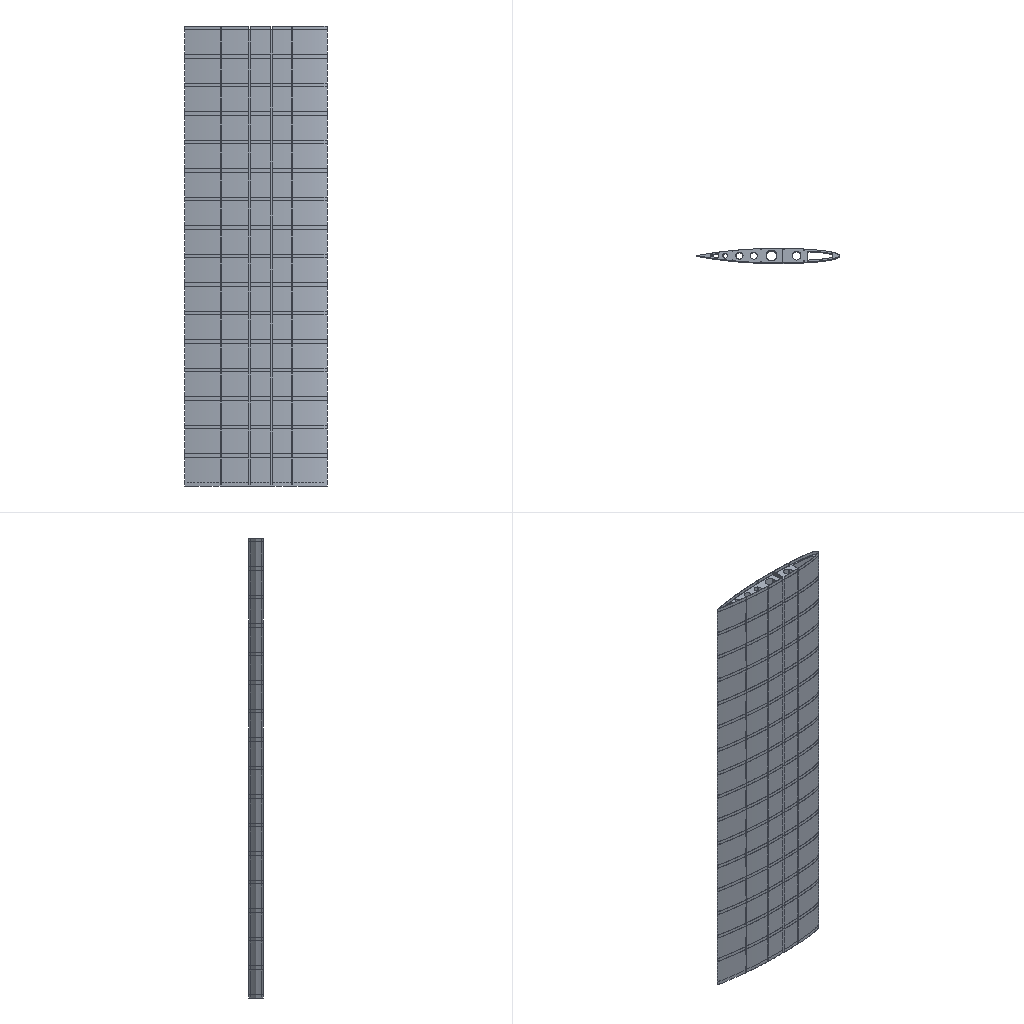Simulation study | abaqus
Set-up summary:
category,name,step,type,value,unit,region
solver,abaqus
solver,version,,,Abaqus/Standard 2020
units,not stated in the deck,,not stated
analysis,deck,,static,static
load_step,Step-1,Step-1,static,nlgeom=True
contact,interactions,,,general=0 pairs=0 ties=0
load_step,requested,,,1
mesh,nodes,,,93184
mesh,elements,,,87242
element_type,S3,,shell,1575
element_type,S4R,,shell,85667
load,load commands in deck,,count,1
bc,support commands in deck,,count,1
material,MATERIAL-1,,in results
check,setup vs results,,match,"per instance, exact: element labels, types and connectivity; labels of the nodes the elements use; coordinates of those nodes at SINGLE_PRECISION in 1 of 1 instance(s)"
Abaqus input file, long lists of numbers shortened:
*Heading
** Job name: Job-2 Model name: Job-15872
** Generated by: Abaqus/CAE 2020
*Preprint, echo=NO, model=NO, history=NO, contact=NO
**
** PARTS
**
*Part, name=PART-4
*Node
      1,  -108.057,  -2.084,           5.
      2,  -110.05,  -1.754,           5.
** (93182 more lines like these left out)
*Element, type=S4R
  1, 58648, 58655, 57835, 57834
  2, 58655, 58656, 57836, 57835
** (85665 more lines like these left out)
*Element, type=S3
271, 90430, 90428, 91111
272, 75408, 75407, 73694
** (1573 more lines like these left out)
*Nset, nset=SET-1
     4,     5,     6,    13,    14,    15,    16,    17,    18,    19,    20,    21,    22,    23,    24,    25
    26,    52,    53,    54,    55,    56,    57,    58,    59,    60,    61,    62,    63,    64,    90,    91
** (2480 more lines like these left out)
*Elset, elset=SET-1
   906,   907,   908,   909,   910,   911,   912,   913,   914,   915,   916,   917,   918,   919,   920,   921
   922,   923,   924,   925,   926,   927,   928,   929,   930,   931,   932,   933,   934,   935,   936,   937
** (2295 more lines like these left out)
*Nset, nset=SET-2
 50078, 50081, 50082, 50090, 50107, 50108, 50110, 50111, 50112, 50121, 50122, 50123, 50223, 50224, 50226, 50227
 50228, 50237, 50238, 50239, 50337, 50338, 50340, 50341, 50342, 50351, 50352, 50353, 50451, 50452, 50454, 50457
** (1104 more lines like these left out)
*Elset, elset=SET-2
   271,   272,   273,   274,   275,   276,   277,   278,   279,   280,   281,   282,   283,   284,   285,   286
   287,   288,   289,   290,   291,   292,   293,   294,   295,   296,   297,   298,   299,   300,   301,   302
** (951 more lines like these left out)
*Nset, nset=SET-8
   622,   636,   660,   705,   737,   773,   805,   841,   880,   909,   948,   977,  1016,  1045,  1091,  1113
  1159,  1181,  1227,  1249,  1302,  1317,  1370,  1385,  1438,  1453,  1513,  1521,  1581,  1589,  1649,  1657
** (317 more lines like these left out)
*Elset, elset=SET-8
   729,   730,   731,   732,   733,   734,   735,   736,   737,   738,   739,   740,   741,   742,   743,   744
   745,   746,   747,   748,   749,   750,   751,   752,   753,   754,   755,   756,   757,   758,   759,   760
** (258 more lines like these left out)
*Nset, nset=SET-9
     1,     2,     3,     4,     5,     6,     7,     8,     9,    10,    11,    12,    13,    14,    15,    16
    17,    27,    28,    29,    30,    31,    32,    33,    34,    35,    36,    37,    38,    39,    40,    41
** (317 more lines like these left out)
*Elset, elset=SET-9
   654,   655,   656,   657,   658,   659,   660,   661,   662,   663,   664,   665,   666,   667,   668,   669
   670,   671,   672,   673,   674,   675,   676,   677,   678,   679,   680,   681,   682,   683,   684,   685
** (258 more lines like these left out)
*Nset, nset=SET-10
 22694, 22695, 22700, 22701, 22702, 22703, 22704, 22705, 22711, 22714, 22715, 22716, 22742, 22747, 22748, 22749
 22750, 22751, 22752, 22753, 22754, 22755, 22756, 22757, 22758, 22759, 22760, 22761, 22762, 22763, 22764, 22765
** (244 more lines like these left out)
*Elset, elset=SET-10
   804,   805,   806,   807,   808,   809,   810,   811,   812,   813,   814,   815,   816,   817,   818,   819
   820,   821,   822,   823,   824,   825,   826,   827,   828,   829,   830,   831,   832,   833,   834,   835
** (197 more lines like these left out)
*Nset, nset=SET-11
 18342, 18343, 18344, 18345, 18346, 18347, 18348, 18349, 18350, 18351, 18352, 18353, 18354, 18355, 18356, 18357
 18358, 18359, 18360, 18361, 18371, 18372, 18373, 18374, 18375, 18376, 18377, 18378, 18379, 18380, 18381, 18382
** (243 more lines like these left out)
*Elset, elset=SET-11
   603,   604,   605,   606,   607,   608,   609,   610,   611,   612,   613,   614,   615,   616,   617,   618
   619,   620,   621,   622,   623,   624,   625,   626,   627,   628,   629,   630,   631,   632,   633,   634
** (197 more lines like these left out)
*Nset, nset=SET-12
 43563, 43564, 43571, 43572, 43573, 43574, 43575, 43576, 43577, 43578, 43579, 43580, 43583, 43584, 43585, 43586
 43587, 43588, 43589, 43590, 43593, 43598, 43599, 43600, 43601, 43602, 43603, 43604, 43605, 43645, 43652, 43653
** (176 more lines like these left out)
*Elset, elset=SET-12
   864,   865,   866,   867,   868,   869,   870,   871,   872,   873,   874,   875,   876,   877,   878,   879
   880,   881,   882,   883,   884,   885,   886,   887,   888,   889,   890,   891,   892,   893,   894,   895
** (141 more lines like these left out)
*Nset, nset=SET-13
 37577, 37578, 37583, 37584, 37585, 37586, 37587, 37588, 37589, 37590, 37591, 37592, 37597, 37598, 37599, 37600
 37601, 37602, 37603, 37604, 37608, 37612, 37613, 37614, 37615, 37616, 37617, 37618, 37619, 37661, 37663, 37664
** (176 more lines like these left out)
*Elset, elset=SET-13
   561,   562,   563,   564,   565,   566,   567,   568,   569,   570,   571,   572,   573,   574,   575,   576
   577,   578,   579,   580,   581,   582,   583,   584,   585,   586,   587,   588,   589,   590,   591,   592
** (141 more lines like these left out)
*Nset, nset=SET-14
 58650, 58651, 58657, 58658, 58659, 58660, 58669, 58670, 58678, 58681, 58682, 58729, 58735, 58736, 58737, 58738
 58739, 58740, 58753, 58754, 58755, 58756, 58757, 58758, 58759, 58760, 58794, 58797, 58798, 58843, 58849, 58850
** (176 more lines like these left out)
*Elset, elset=SET-14
    31,    32,    33,    34,    35,    36,    37,    38,    39,    40,    41,    42,    43,    44,    45,    46
    47,    48,    49,    50,    51,    52,    53,    54,    55,    56,    57,    58,    59,    60,    61,    62
** (141 more lines like these left out)
*Nset, nset=SET-15
 50080, 50081, 50087, 50088, 50089, 50090, 50099, 50100, 50108, 50111, 50112, 50159, 50165, 50166, 50167, 50168
 50169, 50170, 50183, 50184, 50185, 50186, 50187, 50188, 50189, 50190, 50224, 50227, 50228, 50273, 50279, 50280
** (176 more lines like these left out)
*Elset, elset=SET-15
   229,   230,   231,   232,   233,   234,   235,   236,   237,   238,   239,   240,   241,   242,   243,   244
   245,   246,   247,   248,   249,   250,   251,   252,   253,   254,   255,   256,   257,   258,   259,   260
** (141 more lines like these left out)
*Nset, nset=SET-16
 73686, 73687, 73690, 73691, 73692, 73693, 73694, 73695, 73696, 73697, 73700, 73701, 73702, 73703, 73704, 73705
 73706, 73708, 73709, 73710, 73711, 73712, 73713, 73725, 73727, 73728, 73729, 73730, 73731, 73732, 73733, 73734
** (618 more lines like these left out)
*Elset, elset=SET-16
    73,    74,    75,    76,    77,    78,    79,    80,    81,    82,    83,    84,    85,    86,    87,    88
    89,    90,    91,    92,    93,    94,    95,    96,    97,    98,    99,   100,   101,   102,   103,   104
** (508 more lines like these left out)
*Nset, nset=SET-17
 50078, 50079, 50085, 50086, 50107, 50158, 50161, 50162, 50163, 50164, 50223, 50272, 50275, 50276, 50277, 50278
 50337, 50386, 50389, 50390, 50391, 50392, 50451, 50455, 50513, 50516, 50517, 50518, 50565, 50569, 50627, 50630
** (115 more lines like these left out)
*Elset, elset=SET-17
     1,     2,     3,     4,     5,     6,     7,     8,     9,    10,    11,    12,    13,    14,    15,    16
    17,    18,    19,    20,    21,    22,    23,    24,    25,    26,    27,    28,    29,    30,  1387,  1388
** (90 more lines like these left out)
*Nset, nset=SET-18
 50083, 50084, 50091, 50092, 50109, 50113, 50160, 50171, 50172, 50173, 50174, 50175, 50191, 50192, 50193, 50194
 50225, 50229, 50274, 50285, 50286, 50287, 50288, 50289, 50305, 50306, 50307, 50308, 50339, 50343, 50388, 50399
** (127 more lines like these left out)
*Elset, elset=SET-18
   531,   532,   533,   534,   535,   536,   537,   538,   539,   540,   541,   542,   543,   544,   545,   546
   547,   548,   549,   550,   551,   552,   553,   554,   555,   556,   557,   558,   559,   560,  2257,  2258
** (100 more lines like these left out)
*Nset, nset=SET-3
 37578, 37580, 37659, 37660, 37769, 37770, 37879, 37880, 37941, 37942, 38001, 38002, 38111, 38112, 38221, 38222
 38343, 38344, 38381, 38382, 38453, 38454, 38563, 38564, 38685, 38686, 38795, 38796, 38821, 38822, 38905, 38906
** (14 more lines like these left out)
*Elset, elset=SET-3
 86939, 86940, 86941, 86942, 86943, 86944, 86945, 86946, 86947, 86948, 86949, 86950, 86951, 86952, 86953, 86954
 86955, 86956, 86957, 86958, 86959, 86960, 86961, 86962, 86963, 86964, 86965, 86966, 86967, 86968, 86969, 86970
** (7 more lines like these left out)
*Nset, nset=SET-4
 73687, 73689, 73723, 73724, 73781, 73782, 73839, 73840, 73881, 73882, 73905, 73906, 73963, 73964, 74021, 74022
 74087, 74088, 74113, 74114, 74145, 74146, 74203, 74204, 74269, 74270, 74327, 74328, 74345, 74346, 74385, 74386
** (6 more lines like these left out)
*Elset, elset=SET-4
 87003, 87004, 87005, 87006, 87007, 87008, 87009, 87010, 87011, 87012, 87013, 87014, 87015, 87016, 87017, 87018
 87019, 87020, 87021, 87022, 87023, 87024, 87025, 87026, 87027, 87028, 87029, 87030, 87031, 87032, 87033, 87034
** (3 more lines like these left out)
** Section: Section-1-SET-17
*Shell Section, elset=SET-17, material=MATERIAL-1
0.1, 5
** Section: Section-2-SET-14
*Shell Section, elset=SET-14, material=MATERIAL-1
0.1, 5
** Section: Section-3-SET-16
*Shell Section, elset=SET-16, material=MATERIAL-1
0.1, 5
** Section: Section-4-SET-15
*Shell Section, elset=SET-15, material=MATERIAL-1
0.1, 5
** Section: Section-5-SET-2
*Shell Section, elset=SET-2, material=MATERIAL-1
0.1, 5
** Section: Section-6-SET-18
*Shell Section, elset=SET-18, material=MATERIAL-1
0.1, 5
** Section: Section-7-SET-13
*Shell Section, elset=SET-13, material=MATERIAL-1
0.1, 5
** Section: Section-8-SET-11
*Shell Section, elset=SET-11, material=MATERIAL-1
0.1, 5
** Section: Section-9-SET-9
*Shell Section, elset=SET-9, material=MATERIAL-1
0.1, 5
** Section: Section-10-SET-8
*Shell Section, elset=SET-8, material=MATERIAL-1
0.1, 5
** Section: Section-11-SET-10
*Shell Section, elset=SET-10, material=MATERIAL-1
0.1, 5
** Section: Section-12-SET-12
*Shell Section, elset=SET-12, material=MATERIAL-1
0.1, 5
** Section: Section-13-SET-1
*Shell Section, elset=SET-1, material=MATERIAL-1
0.1, 5
** Section: Section-14-SET-3
*Shell Section, elset=SET-3, material=MATERIAL-1
0.5755, 5
** Section: Section-15-SET-4
*Shell Section, elset=SET-4, material=MATERIAL-1
0.4965, 5
*End Part
**
**
** ASSEMBLY
**
*Assembly, name=Assembly
**
*Instance, name=PART-4-2, part=PART-4
*End Instance
**
*Node
      1,           0.,          10.,         645.
      2,           0.,          10.,           0.
** (5 more lines like these left out)
*Nset, nset=SET-3, instance=PART-4-2
   584,   585,   586,   587,   588,   589,   590,   591,   592,   593,   594,   595,   596,   597,   598,   599
   600,   601,   602,   603,   604,   605,   606,   607,   608,   609,   610,   611,   612,   613,  1657,  1658
** (301 more lines like these left out)
*Nset, nset=Set-4, instance=PART-4-2
   589,   590,   591,   592,   593,  1657,  1665,  1666,  1667,  1668,  1669,  1670,  1671,  1700,  1701,  1702
  1703,  1704,  1705,  1706,  1707,  1708,  1709,  2773,  2774,  2775,  2776,  2777,  2778,  2779,  2808,  2809
** (176 more lines like these left out)
*Nset, nset=Set-5
 2,
*Nset, nset=Set-6, instance=PART-4-2
   584,   585,   586,   587,   588,   594,   595,   596,   597,   598,   599,   600,   601,   602,   603,   604
   605,   606,   607,   608,   609,   610,   611,   612,   613,  1658,  1659,  1660,  1661,  1662,  1663,  1664
** (135 more lines like these left out)
*Nset, nset=Set-6
 1, 3, 4, 5, 6, 7
*Nset, nset=Set-7, instance=PART-4-2
   589,   590,   591,   592,   593,  1657,  1665,  1666,  1667,  1668,  1669,  1670,  1671,  1700,  1701,  1702
  1703,  1704,  1705,  1706,  1707,  1708,  1709,  2773,  2774,  2775,  2776,  2777,  2778,  2779,  2808,  2809
** (176 more lines like these left out)
*Nset, nset=Set-8, instance=PART-4-2
   589,   590,   591,   592,   593,  1657,  1665,  1666,  1667,  1668,  1669,  1670,  1671,  1700,  1701,  1702
  1703,  1704,  1705,  1706,  1707,  1708,  1709,  2773,  2774,  2775,  2776,  2777,  2778,  2779,  2808,  2809
** (176 more lines like these left out)
*Nset, nset=_PICKEDSET246, internal
 2,
*Elset, elset=__PICKEDSURF245_SPOS, internal, instance=PART-4-2
    1,    2,    3,    4,    5,    6,    7,    8,    9,   10,   11,   12,   13,   14,   15,   16
   17,   18,   19,   20,   21,   22,   23,   24,   25,   26,   27,   28,   29,   30,  271,  272
** (47 more lines like these left out)
*Surface, type=ELEMENT, name=_PICKEDSURF245, internal
__PICKEDSURF245_SPOS, SPOS
** Constraint: CONSTRAINT-2
*Coupling, constraint name=CONSTRAINT-2, ref node=_PICKEDSET246, surface=_PICKEDSURF245
*Kinematic
*End Assembly
*Amplitude, name=Amp-1
             0.,              0.,              1.,              1.
**
** MATERIALS
**
*Material, name=MATERIAL-1
*Density
 2.4e-09,
*Elastic
27000., 0.3
** ----------------------------------------------------------------
**
** STEP: Step-1
**
*Step, name=Step-1, nlgeom=YES
*Static
0.01, 1., 1e-05, 0.1
**
** BOUNDARY CONDITIONS
**
** Name: BC-1 Type: 对称/反对称/完全固定
*Boundary
Set-8, ENCASTRE
**
** LOADS
**
** Name: Load-1   Type: Concentrated force
*Cload
Set-5, 2, 0.5
**
** OUTPUT REQUESTS
**
*Restart, write, frequency=0
**
** FIELD OUTPUT: F-Output-1
**
*Output, field, variable=PRESELECT
**
** HISTORY OUTPUT: H-Output-1
**
*Output, history, variable=PRESELECT
*End Step
Results summary:
result,step,,completed,increments=15 time=1.0/1.0
result,analysis,,,static
result,last_loadstep,,,1
result,analysis steps,,count,1
result,primary field,,,"U, UR"
result,reaction total,,FX,0.0,model units
result,reaction total,,FY,-0.5,model units
result,reaction total,,FZ,-1e-06,model units